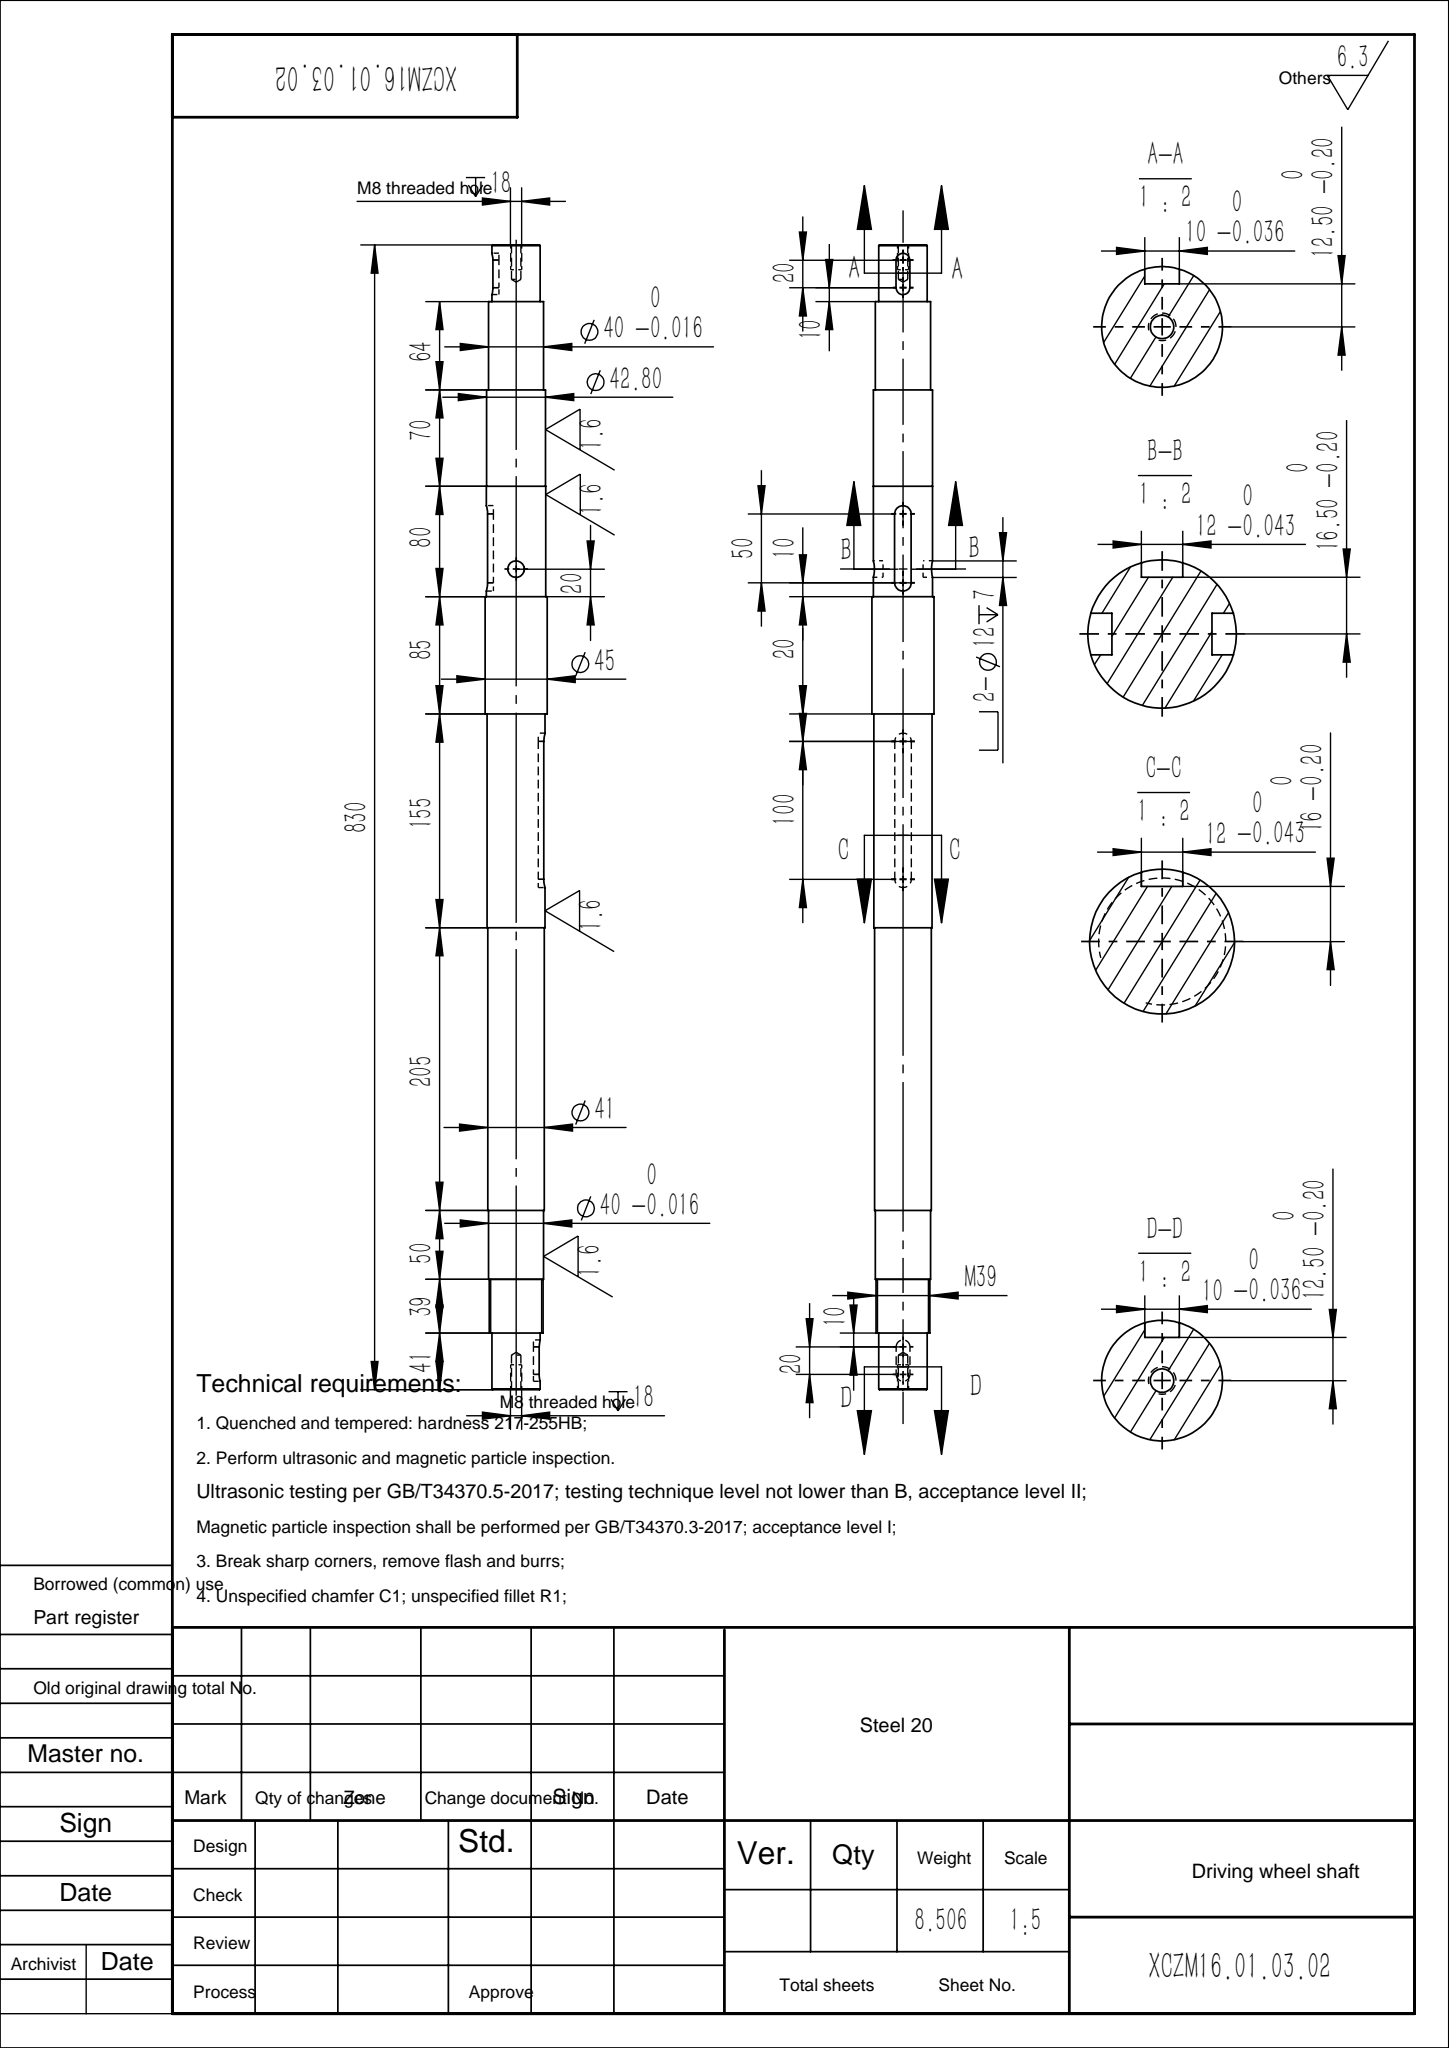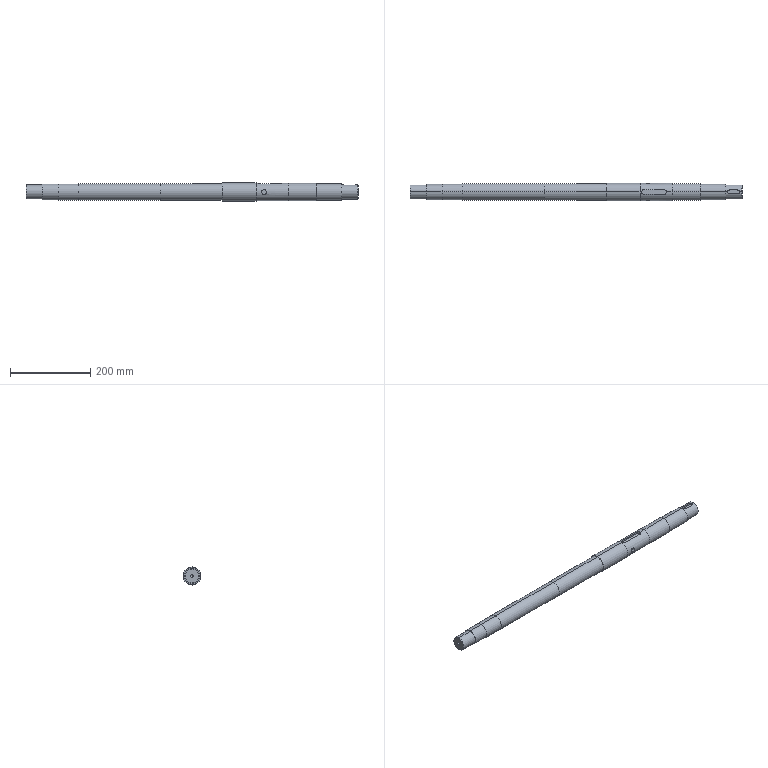Part | SolidWorks | features ICE 5, HoleWzd 2, Chamfer 1, MirrorPattern 1, Revolution 1 | 1 solid | 73 faces | box 830 x 45 x 45 mm | volume 1090554 mm3 | cylinder 40 | plane 25 | cone 8 | commonest cylinder face diameters 12 x10 10 x6 6.8 x4 35 x4 40 x4 39 x2